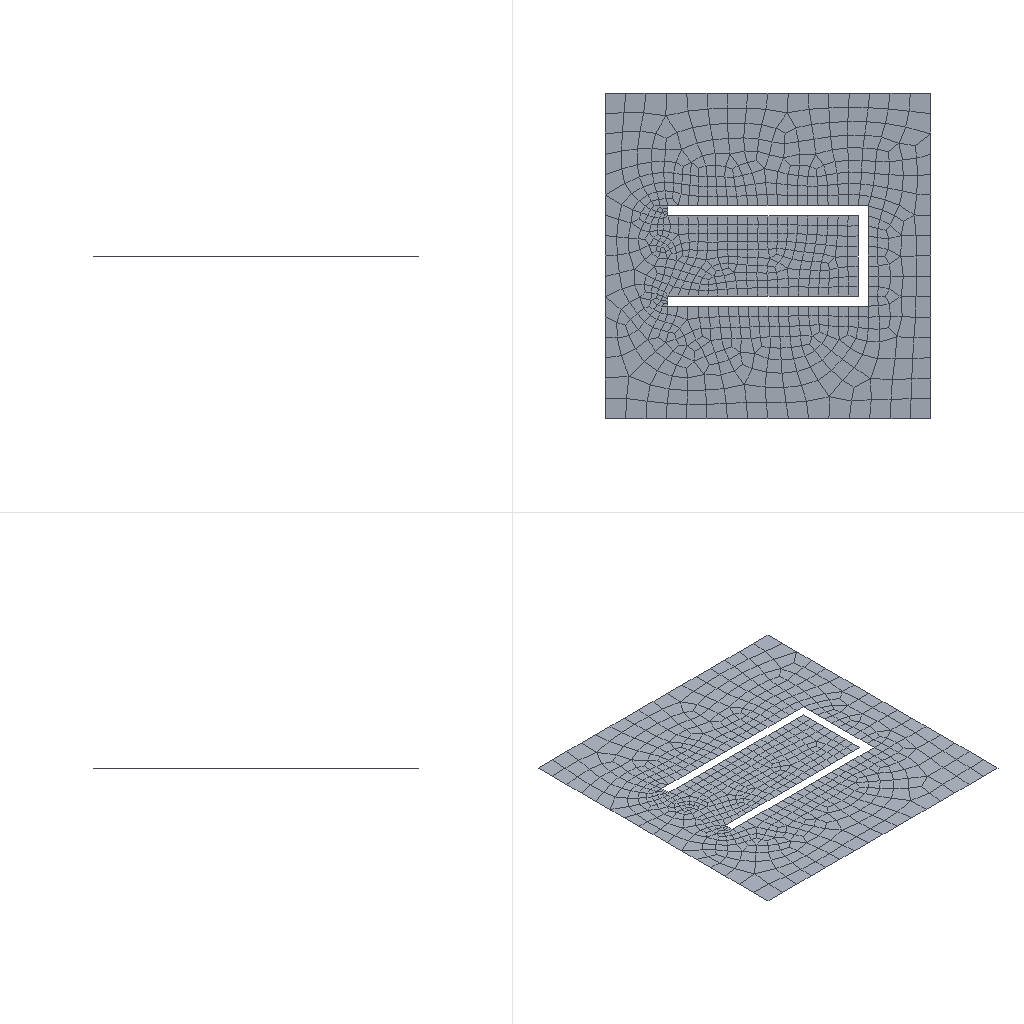Simulation study | abaqus
Set-up summary:
category,name,step,type,value,unit,region
solver,abaqus
solver,version,,,Abaqus/Explicit 2020
units,not stated in the deck,,not stated
analysis,deck,,transient,transient
load_step,Step-u,Step-u,transient
load_step,Step-1,Step-1,transient
load_step,requested,,,2
mesh,nodes,,,1651
mesh,elements,,,1447
element_type,S4R,,shell,732
element_type,MASS,,point,3
element_type,R3D3,,rigid,6
element_type,R3D4,,rigid,703
element_type,ROTARYI,,mass,3
load,load commands in deck,,count,2
bc,support commands in deck,,count,14
material,CHUNTIE N,,in results
check,setup vs results,,match,"per instance, exact: element labels, types and connectivity; labels of the nodes the elements use; coordinates of those nodes at SINGLE_PRECISION in 4 of 4 instance(s)"
Abaqus input file, long lists of numbers shortened:
*Heading
** Job name: Job-2 Model name: Model-1
** Generated by: Abaqus/CAE 2020
*Preprint, echo=NO, model=NO, history=NO, contact=NO
**
** PARTS
**
*Part, name=blank
*Node
      1,        1.625,       -1.625,   -2.15
      2,       -1.625,       -1.625,   -2.15
** (814 more lines like these left out)
*Element, type=S4R
  1, 700, 710, 721, 713
  2, 377, 190, 284, 454
** (730 more lines like these left out)
*Nset, nset=Set-1, generate
   1,  816,    1
*Elset, elset=Set-1, generate
   1,  732,    1
** Section: Section-1
*Shell Section, elset=Set-1, material="chuntie n"
0.3, 5
*End Part
**
*Part, name=flange
*Node
      1, -0.8958, -0.4,  -1.009
      2,          -1., -0.4,          -1.
** (394 more lines like these left out)
*Element, type=R3D4
 1,   1,  11, 118,  36
 2,  11,  12, 119, 118
** (348 more lines like these left out)
*Node
    397,  0.8738,           0.,  -1.305
*Nset, nset=flange-RefPt_, internal
397,
*Nset, nset=Set-7
 397,
*Elset, elset=flange, generate
   1,  350,    1
*Element, type=MASS, elset=Set-7_Inertia-1_MASS_
351, 397
*Mass, elset=Set-7_Inertia-1_MASS_
1.,
*Element, type=ROTARYI, elset=Set-7_Inertia-1_ROTI_
352, 397
*Rotary Inertia, elset=Set-7_Inertia-1_ROTI_
1., 1., 1., 0., 0., 0.
*End Part
**
*Part, name=pad
*Node
      1,         1.75,        -1.75,  -1.67
      2,        -1.75,        -1.75,  -1.67
** (172 more lines like these left out)
*Element, type=R3D3
1, 163,  84,  85
2, 164, 102, 103
** (2 more lines like these left out)
*Element, type=R3D4
  5,  69,  20,  21,  83
  6,  21,  22,  84,  83
** (136 more lines like these left out)
*Node
    175,        -1.75,           0.,  -1.67
*Nset, nset=pad-RefPt_, internal
175,
*Nset, nset=Set-3
 175,
*Elset, elset=pad, generate
   1,  142,    1
*Element, type=MASS, elset=Set-3_Inertia-1_MASS_
143, 175
*Mass, elset=Set-3_Inertia-1_MASS_
1.,
*Element, type=ROTARYI, elset=Set-3_Inertia-1_ROTI_
144, 175
*Rotary Inertia, elset=Set-3_Inertia-1_ROTI_
1., 1., 1., 0., 0., 0.
*End Part
**
*Part, name=post
*Node
      1,  -0.9479,  0.4,  -2.305
      2,  -0.9479, -0.4,  -2.305
** (260 more lines like these left out)
*Element, type=R3D4
1,  1, 19, 22,  4
2, 19, 20, 21, 22
** (213 more lines like these left out)
*Element, type=R3D3
28, 131, 230, 186
29, 228, 184, 133
*Node
    263,          -2.,           0.,  -2.3
*Nset, nset=post-RefPt_, internal
263,
*Nset, nset=Set-5
 263,
*Elset, elset=post, generate
   1,  217,    1
*Element, type=MASS, elset=Set-5_Inertia-1_MASS_
218, 263
*Mass, elset=Set-5_Inertia-1_MASS_
1.,
*Element, type=ROTARYI, elset=Set-5_Inertia-1_ROTI_
219, 263
*Rotary Inertia, elset=Set-5_Inertia-1_ROTI_
1., 1., 1., 0., 0., 0.
*End Part
**
**
** ASSEMBLY
**
*Assembly, name=Assembly
**
*Instance, name=post-1, part=post
*End Instance
**
*Instance, name=flange-1, part=flange
          0.,           0.,         -0.5
*End Instance
**
*Instance, name=pad-1, part=pad
          0.,           0., -0.33
*End Instance
**
*Instance, name=blank-1, part=blank
*End Instance
**
*Nset, nset=Set-1, instance=blank-1, generate
   1,  816,    1
*Elset, elset=Set-1, instance=blank-1, generate
   1,  732,    1
*Nset, nset=Set-2, instance=pad-1, generate
   1,  174,    1
*Elset, elset=Set-2, instance=pad-1, generate
   1,  142,    1
*Nset, nset=Set-7, instance=post-1
 263,
*Nset, nset=Set-8, instance=pad-1
 175,
*Nset, nset=Set-9, instance=pad-1
 175,
*Nset, nset=Set-10, instance=flange-1
 397,
*Nset, nset=Set-11, instance=blank-1
  1,  2,  3,  4, 13, 14, 15, 16, 17, 18, 19, 20, 21, 22, 23, 24
 25, 26, 27, 28, 29, 30, 31, 32, 33, 34, 35, 36, 37, 38, 39, 40
** (2 more lines like these left out)
*Elset, elset=Set-11, instance=blank-1
  25,  36,  50,  61,  63, 391, 395, 397, 410, 525, 527, 534, 539, 546, 553, 561
 569, 588, 595, 596, 597, 603, 609, 610, 611, 621, 623, 628, 632, 634, 639, 640
** (2 more lines like these left out)
*Nset, nset=Set-12, instance=blank-1
  1,  2,  3,  4, 13, 14, 15, 16, 17, 18, 19, 20, 21, 22, 23, 24
 25, 26, 27, 43, 44, 45, 46, 47, 48, 49, 50, 51, 52, 53, 54, 55
** (2 more lines like these left out)
*Elset, elset=Set-12, instance=blank-1
  25,  36,  50,  61,  63, 391, 395, 397, 410, 539, 546, 561, 588, 595, 596, 597
 603, 621, 623, 632, 634, 639, 641, 644, 645, 649, 652, 653, 663, 670, 671, 673
** (1 more lines like these left out)
*Elset, elset=_m_Surf-1_SPOS, internal, instance=pad-1, generate
   1,  142,    1
*Surface, type=ELEMENT, name=m_Surf-1
_m_Surf-1_SPOS, SPOS
*Elset, elset=_m_Surf-3_SPOS, internal, instance=flange-1, generate
   1,  350,    1
*Surface, type=ELEMENT, name=m_Surf-3
_m_Surf-3_SPOS, SPOS
*Elset, elset=_m_Surf-5_SNEG, internal, instance=post-1, generate
   1,  217,    1
*Surface, type=ELEMENT, name=m_Surf-5
_m_Surf-5_SNEG, SNEG
*Elset, elset=_s_Surf-1_SNEG, internal, instance=blank-1, generate
   1,  732,    1
*Surface, type=ELEMENT, name=s_Surf-1
_s_Surf-1_SNEG, SNEG
*Elset, elset=_s_Surf-3_SNEG, internal, instance=blank-1, generate
   1,  732,    1
*Surface, type=ELEMENT, name=s_Surf-3
_s_Surf-3_SNEG, SNEG
*Elset, elset=_s_Surf-5_SPOS, internal, instance=blank-1, generate
   1,  732,    1
*Surface, type=ELEMENT, name=s_Surf-5
_s_Surf-5_SPOS, SPOS
*Rigid Body, ref node=post-1.post-RefPt_, elset=post-1.post
*Rigid Body, ref node=flange-1.flange-RefPt_, elset=flange-1.flange
*Rigid Body, ref node=pad-1.pad-RefPt_, elset=pad-1.pad
*End Assembly
**
** MATERIALS
**
*Material, name="chuntie n"
*Density
 7.875e-09,
*Elastic
80650., 0.291
*Plastic
   98.45,   0.
 207.085, 0.02
 222.526, 0.04
 232.557, 0.06
 240.162, 0.08
 246.357,  0.1
 251.619, 0.12
 256.214, 0.14
 260.305, 0.16
  267.38,  0.2
 281.038,  0.3
 291.392,  0.4
 299.826,  0.5
  306.99,  0.6
**
** INTERACTION PROPERTIES
**
*Surface Interaction, name=IntProp-1
*Friction
 0.2,
*Surface Behavior, pressure-overclosure=HARD
**
** BOUNDARY CONDITIONS
**
** Name: BC-1 Type: 对称/反对称/完全固定
*Boundary
Set-7, ENCASTRE
** ----------------------------------------------------------------
**
** STEP: Step-u
**
*Step, name=Step-u, nlgeom=YES
*Dynamic, Explicit
, 0.001
*Bulk Viscosity
0.06, 1.2
**
** BOUNDARY CONDITIONS
**
** Name: [REDACTED] : Velocity/Angular velocity
*Boundary, type=VELOCITY
Set-9, 1, 1
Set-9, 2, 2
Set-9, 3, 3, -149.
Set-9, 4, 4
Set-9, 5, 5
Set-9, 6, 6
**
** OUTPUT REQUESTS
**
*Restart, write, number interval=1, time marks=NO
**
** FIELD OUTPUT: F-Output-1
**
*Output, field, number interval=50
*Node Output
A, RF, U, V
*Element Output, directions=YES
E, EVF, LE, MISES, PE, PEEQ, PEEQVAVG, PEVAVG, S, SSAVG, SVAVG
*Contact Output
CSTRESS,
*Output, history, frequency=0
*End Step
** ----------------------------------------------------------------
**
** STEP: Step-1
**
*Step, name=Step-1, nlgeom=YES
*Dynamic, Explicit
, 0.001
*Bulk Viscosity
0.06, 1.2
**
** BOUNDARY CONDITIONS
**
** Name: BC-3 Type: 速度/角速度
*Boundary, type=VELOCITY
Set-10, 1, 1
Set-10, 2, 2
Set-10, 3, 3, -800.
Set-10, 4, 4
Set-10, 5, 5
Set-10, 6, 6
** Name: [REDACTED] : Velocity/Angular velocity
*Boundary, type=VELOCITY
Set-9, 3, 3
**
** INTERACTIONS
**
** Interaction: Int-1
*Contact, op=NEW
*Contact Inclusions, ALL EXTERIOR
*Contact Property Assignment
 ,  , IntProp-1
**
** OUTPUT REQUESTS
**
*Restart, write, number interval=1, time marks=NO
**
** FIELD OUTPUT: F-Output-1
**
*Output, field, number interval=50
*Node Output
A, RF, U, V
*Element Output, directions=YES
E, EVF, LE, MISES, PE, PEEQ, PEEQVAVG, PEVAVG, S, SSAVG, SVAVG
*Contact Output
CSTRESS,
**
** HISTORY OUTPUT: H-Output-1
**
*Output, history, variable=PRESELECT
*End Step
Results summary:
result,step,Step-u,completed,increments=160166 time=0.001/0.001
result,step,Step-1,completed,increments=158146 time=0.001/0.001
result,analysis,,,transient
result,last_loadstep,,,2
result,primary field,,,"U, UR"
result,reaction total,,FX,-2097152.0,model units
result,reaction total,,FY,-79.262,model units
result,reaction total,,FZ,7516192768.0,model units